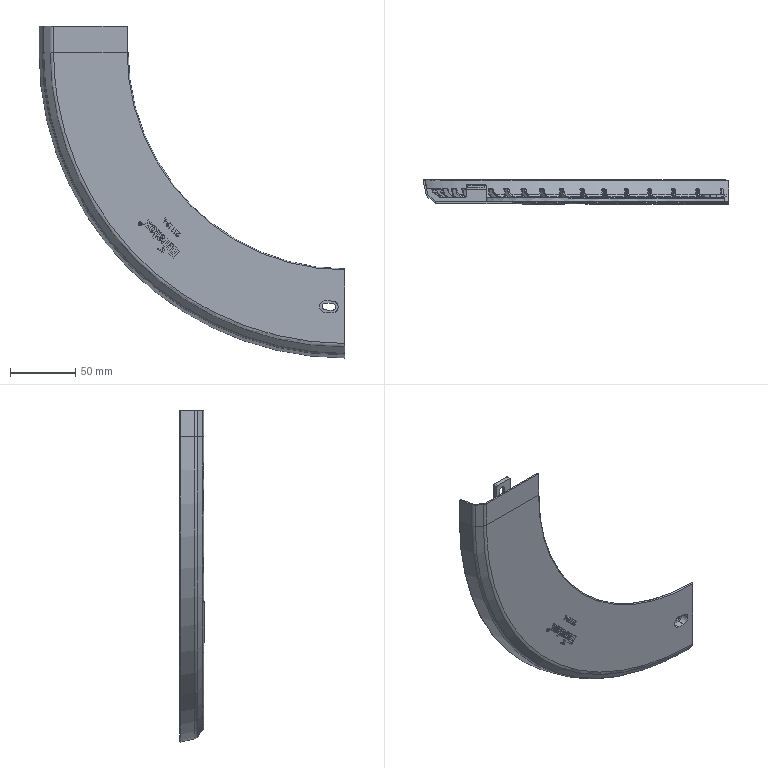Part | STEP file | V00-000000454 | 2 solids | 2029 faces | box 234.244 x 18.951 x 254.244 mm | volume 49218 mm3 | cylinder 669 | torus 480 | plane 362 | spline 254 | sphere 241 | cone 23 | commonest cylinder face diameters 1 x512 2 x44 1.048 x20 420 x19 423 x19 375 x18